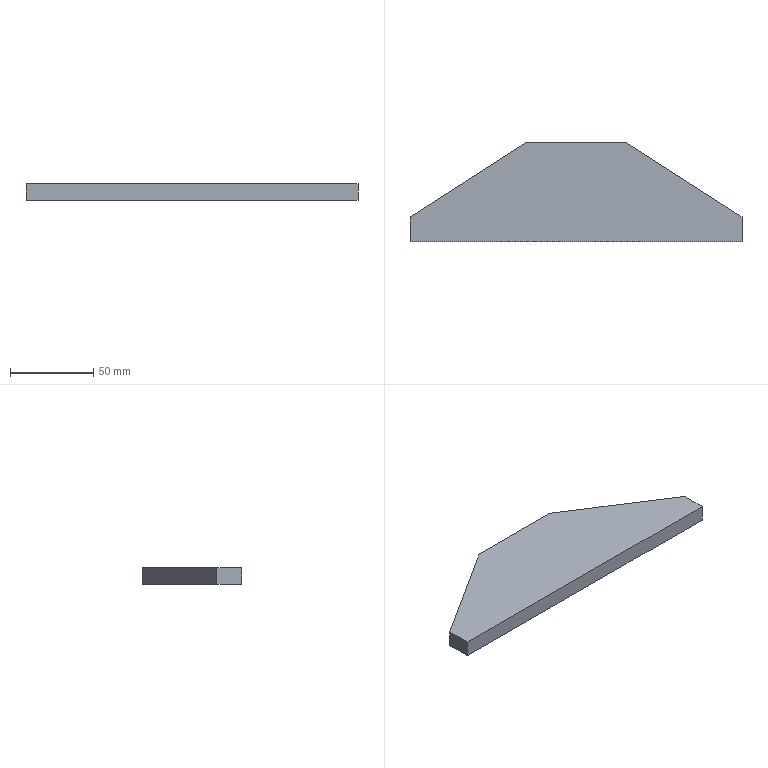Part | SolidWorks | features BaseBody 1 | 1 solid | 8 faces | box 200 x 60 x 10 mm | volume 88500 mm3 | plane 8
STEP:
#1=CARTESIAN_POINT('',(100.,-60.,-5.));
#2=VERTEX_POINT('',#1);
#3=CARTESIAN_POINT('',(100.,-45.,-5.));
#4=VERTEX_POINT('',#3);
#5=CARTESIAN_POINT('',(100.,-45.,-5.));
#6=DIRECTION('',(0.,1.,0.));
#7=VECTOR('',#6,1000.);
#8=LINE('',#5,#7);
#9=EDGE_CURVE('',#2,#4,#8,.T.);
#10=ORIENTED_EDGE('',*,*,#9,.F.);
#11=CARTESIAN_POINT('',(-100.,-60.,-5.));
#12=VERTEX_POINT('',#11);
#13=CARTESIAN_POINT('',(-100.,-60.,-5.));
#14=DIRECTION('',(1.,0.,0.));
#15=VECTOR('',#14,1000.);
#16=LINE('',#13,#15);
#17=EDGE_CURVE('',#12,#2,#16,.T.);
#18=ORIENTED_EDGE('',*,*,#17,.F.);
#19=CARTESIAN_POINT('',(-100.,-45.,-5.));
#20=VERTEX_POINT('',#19);
#21=CARTESIAN_POINT('',(-100.,-45.,-5.));
#22=DIRECTION('',(0.,-1.,0.));
#23=VECTOR('',#22,1000.);
#24=LINE('',#21,#23);
#25=EDGE_CURVE('',#20,#12,#24,.T.);
#26=ORIENTED_EDGE('',*,*,#25,.F.);
#27=CARTESIAN_POINT('',(-30.,0.,-5.));
#28=VERTEX_POINT('',#27);
#29=CARTESIAN_POINT('',(-30.,0.,-5.));
#30=DIRECTION('',(-0.8412,-0.5408,0.));
#31=VECTOR('',#30,1000.);
#32=LINE('',#29,#31);
#33=EDGE_CURVE('',#28,#20,#32,.T.);
#34=ORIENTED_EDGE('',*,*,#33,.F.);
#35=CARTESIAN_POINT('',(30.,0.,-5.));
#36=VERTEX_POINT('',#35);
#37=CARTESIAN_POINT('',(-30.,0.,-5.));
#38=DIRECTION('',(-1.,0.,0.));
#39=VECTOR('',#38,1000.);
#40=LINE('',#37,#39);
#41=EDGE_CURVE('',#36,#28,#40,.T.);
#42=ORIENTED_EDGE('',*,*,#41,.F.);
#43=CARTESIAN_POINT('',(30.,0.,-5.));
#44=DIRECTION('',(-0.8412,0.5408,0.));
#45=VECTOR('',#44,1000.);
#46=LINE('',#43,#45);
#47=EDGE_CURVE('',#4,#36,#46,.T.);
#48=ORIENTED_EDGE('',*,*,#47,.F.);
#49=EDGE_LOOP('',(#10,#18,#26,#34,#42,#48));
#50=FACE_OUTER_BOUND('',#49,.T.);
#51=CARTESIAN_POINT('',(0.,0.,-5.));
#52=DIRECTION('',(0.,0.,1.));
#53=DIRECTION('',(1.,0.,0.));
#54=AXIS2_PLACEMENT_3D('',#51,#52,#53);
#55=PLANE('',#54);
#56=ADVANCED_FACE('',(#50),#55,.F.);
#57=CARTESIAN_POINT('',(100.,-60.,5.));
#58=VERTEX_POINT('',#57);
#59=CARTESIAN_POINT('',(100.,-45.,5.));
#60=VERTEX_POINT('',#59);
#61=CARTESIAN_POINT('',(100.,-45.,5.));
#62=DIRECTION('',(0.,1.,0.));
#63=VECTOR('',#62,1000.);
#64=LINE('',#61,#63);
#65=EDGE_CURVE('',#58,#60,#64,.T.);
#66=ORIENTED_EDGE('',*,*,#65,.T.);
#67=CARTESIAN_POINT('',(30.,0.,5.));
#68=VERTEX_POINT('',#67);
#69=CARTESIAN_POINT('',(30.,0.,5.));
#70=DIRECTION('',(-0.8412,0.5408,0.));
#71=VECTOR('',#70,1000.);
#72=LINE('',#69,#71);
#73=EDGE_CURVE('',#60,#68,#72,.T.);
#74=ORIENTED_EDGE('',*,*,#73,.T.);
#75=CARTESIAN_POINT('',(-30.,0.,5.));
#76=VERTEX_POINT('',#75);
#77=CARTESIAN_POINT('',(-30.,0.,5.));
#78=DIRECTION('',(-1.,0.,0.));
#79=VECTOR('',#78,1000.);
#80=LINE('',#77,#79);
#81=EDGE_CURVE('',#68,#76,#80,.T.);
#82=ORIENTED_EDGE('',*,*,#81,.T.);
#83=CARTESIAN_POINT('',(-100.,-45.,5.));
#84=VERTEX_POINT('',#83);
#85=CARTESIAN_POINT('',(-30.,0.,5.));
#86=DIRECTION('',(-0.8412,-0.5408,0.));
#87=VECTOR('',#86,1000.);
#88=LINE('',#85,#87);
#89=EDGE_CURVE('',#76,#84,#88,.T.);
#90=ORIENTED_EDGE('',*,*,#89,.T.);
#91=CARTESIAN_POINT('',(-100.,-60.,5.));
#92=VERTEX_POINT('',#91);
#93=CARTESIAN_POINT('',(-100.,-45.,5.));
#94=DIRECTION('',(0.,-1.,0.));
#95=VECTOR('',#94,1000.);
#96=LINE('',#93,#95);
#97=EDGE_CURVE('',#84,#92,#96,.T.);
#98=ORIENTED_EDGE('',*,*,#97,.T.);
#99=CARTESIAN_POINT('',(-100.,-60.,5.));
#100=DIRECTION('',(1.,0.,0.));
#101=VECTOR('',#100,1000.);
#102=LINE('',#99,#101);
#103=EDGE_CURVE('',#92,#58,#102,.T.);
#104=ORIENTED_EDGE('',*,*,#103,.T.);
#105=EDGE_LOOP('',(#66,#74,#82,#90,#98,#104));
#106=FACE_OUTER_BOUND('',#105,.T.);
#107=CARTESIAN_POINT('',(0.,0.,5.));
#108=DIRECTION('',(0.,0.,1.));
#109=DIRECTION('',(1.,0.,0.));
#110=AXIS2_PLACEMENT_3D('',#107,#108,#109);
#111=PLANE('',#110);
#112=ADVANCED_FACE('',(#106),#111,.T.);
#113=ORIENTED_EDGE('',*,*,#17,.T.);
#114=CARTESIAN_POINT('',(100.,-60.,5.));
#115=DIRECTION('',(0.,0.,-1.));
#116=VECTOR('',#115,1000.);
#117=LINE('',#114,#116);
#118=EDGE_CURVE('',#58,#2,#117,.T.);
#119=ORIENTED_EDGE('',*,*,#118,.F.);
#120=ORIENTED_EDGE('',*,*,#103,.F.);
#121=CARTESIAN_POINT('',(-100.,-60.,5.));
#122=DIRECTION('',(0.,0.,-1.));
#123=VECTOR('',#122,1000.);
#124=LINE('',#121,#123);
#125=EDGE_CURVE('',#92,#12,#124,.T.);
#126=ORIENTED_EDGE('',*,*,#125,.T.);
#127=EDGE_LOOP('',(#113,#119,#120,#126));
#128=FACE_OUTER_BOUND('',#127,.T.);
#129=CARTESIAN_POINT('',(-100.,-60.,5.));
#130=DIRECTION('',(0.,1.,0.));
#131=DIRECTION('',(1.,0.,0.));
#132=AXIS2_PLACEMENT_3D('',#129,#130,#131);
#133=PLANE('',#132);
#134=ADVANCED_FACE('',(#128),#133,.F.);
#135=ORIENTED_EDGE('',*,*,#25,.T.);
#136=ORIENTED_EDGE('',*,*,#125,.F.);
#137=ORIENTED_EDGE('',*,*,#97,.F.);
#138=CARTESIAN_POINT('',(-100.,-45.,5.));
#139=DIRECTION('',(0.,0.,-1.));
#140=VECTOR('',#139,1000.);
#141=LINE('',#138,#140);
#142=EDGE_CURVE('',#84,#20,#141,.T.);
#143=ORIENTED_EDGE('',*,*,#142,.T.);
#144=EDGE_LOOP('',(#135,#136,#137,#143));
#145=FACE_OUTER_BOUND('',#144,.T.);
#146=CARTESIAN_POINT('',(-100.,-45.,5.));
#147=DIRECTION('',(1.,0.,0.));
#148=DIRECTION('',(0.,1.,0.));
#149=AXIS2_PLACEMENT_3D('',#146,#147,#148);
#150=PLANE('',#149);
#151=ADVANCED_FACE('',(#145),#150,.F.);
#152=ORIENTED_EDGE('',*,*,#33,.T.);
#153=ORIENTED_EDGE('',*,*,#142,.F.);
#154=ORIENTED_EDGE('',*,*,#89,.F.);
#155=CARTESIAN_POINT('',(-30.,0.,5.));
#156=DIRECTION('',(0.,0.,-1.));
#157=VECTOR('',#156,1000.);
#158=LINE('',#155,#157);
#159=EDGE_CURVE('',#76,#28,#158,.T.);
#160=ORIENTED_EDGE('',*,*,#159,.T.);
#161=EDGE_LOOP('',(#152,#153,#154,#160));
#162=FACE_OUTER_BOUND('',#161,.T.);
#163=CARTESIAN_POINT('',(-30.,0.,5.));
#164=DIRECTION('',(0.5408,-0.8412,0.));
#165=DIRECTION('',(0.,0.,-1.));
#166=AXIS2_PLACEMENT_3D('',#163,#164,#165);
#167=PLANE('',#166);
#168=ADVANCED_FACE('',(#162),#167,.F.);
#169=ORIENTED_EDGE('',*,*,#41,.T.);
#170=ORIENTED_EDGE('',*,*,#159,.F.);
#171=ORIENTED_EDGE('',*,*,#81,.F.);
#172=CARTESIAN_POINT('',(30.,0.,5.));
#173=DIRECTION('',(0.,0.,-1.));
#174=VECTOR('',#173,1000.);
#175=LINE('',#172,#174);
#176=EDGE_CURVE('',#68,#36,#175,.T.);
#177=ORIENTED_EDGE('',*,*,#176,.T.);
#178=EDGE_LOOP('',(#169,#170,#171,#177));
#179=FACE_OUTER_BOUND('',#178,.T.);
#180=CARTESIAN_POINT('',(-30.,0.,5.));
#181=DIRECTION('',(0.,-1.,0.));
#182=DIRECTION('',(0.,0.,-1.));
#183=AXIS2_PLACEMENT_3D('',#180,#181,#182);
#184=PLANE('',#183);
#185=ADVANCED_FACE('',(#179),#184,.F.);
#186=ORIENTED_EDGE('',*,*,#47,.T.);
#187=ORIENTED_EDGE('',*,*,#176,.F.);
#188=ORIENTED_EDGE('',*,*,#73,.F.);
#189=CARTESIAN_POINT('',(100.,-45.,5.));
#190=DIRECTION('',(0.,0.,-1.));
#191=VECTOR('',#190,1000.);
#192=LINE('',#189,#191);
#193=EDGE_CURVE('',#60,#4,#192,.T.);
#194=ORIENTED_EDGE('',*,*,#193,.T.);
#195=EDGE_LOOP('',(#186,#187,#188,#194));
#196=FACE_OUTER_BOUND('',#195,.T.);
#197=CARTESIAN_POINT('',(30.,0.,5.));
#198=DIRECTION('',(-0.5408,-0.8412,0.));
#199=DIRECTION('',(-0.8412,0.5408,0.));
#200=AXIS2_PLACEMENT_3D('',#197,#198,#199);
#201=PLANE('',#200);
#202=ADVANCED_FACE('',(#196),#201,.F.);
#203=ORIENTED_EDGE('',*,*,#9,.T.);
#204=ORIENTED_EDGE('',*,*,#193,.F.);
#205=ORIENTED_EDGE('',*,*,#65,.F.);
#206=ORIENTED_EDGE('',*,*,#118,.T.);
#207=EDGE_LOOP('',(#203,#204,#205,#206));
#208=FACE_OUTER_BOUND('',#207,.T.);
#209=CARTESIAN_POINT('',(100.,-45.,5.));
#210=DIRECTION('',(-1.,0.,0.));
#211=DIRECTION('',(0.,0.,1.));
#212=AXIS2_PLACEMENT_3D('',#209,#210,#211);
#213=PLANE('',#212);
#214=ADVANCED_FACE('',(#208),#213,.F.);
#215=CLOSED_SHELL('',(#56,#112,#134,#151,#168,#185,#202,#214));
#216=MANIFOLD_SOLID_BREP('',#215);
#217=CARTESIAN_POINT('',(0.,0.,0.));
#218=DIRECTION('',(0.,0.,1.));
#219=DIRECTION('',(1.,0.,0.));
#220=AXIS2_PLACEMENT_3D('',#217,#218,#219);
#221=(LENGTH_UNIT()NAMED_UNIT(*)SI_UNIT(.MILLI.,.METRE.));
#222=UNCERTAINTY_MEASURE_WITH_UNIT(LENGTH_MEASURE(0.00001),#221,'','');
#223=(NAMED_UNIT(*)PLANE_ANGLE_UNIT()SI_UNIT($,.RADIAN.));
#224=(NAMED_UNIT(*)SI_UNIT($,.STERADIAN.)SOLID_ANGLE_UNIT());
#225=(GEOMETRIC_REPRESENTATION_CONTEXT(3)GLOBAL_UNCERTAINTY_ASSIGNED_CONTEXT((#222))GLOBAL_UNIT_ASSIGNED_CONTEXT((#221,#223,#224))REPRESENTATION_CONTEXT('',''));
#226=ADVANCED_BREP_SHAPE_REPRESENTATION('',(#216,#220),#225);